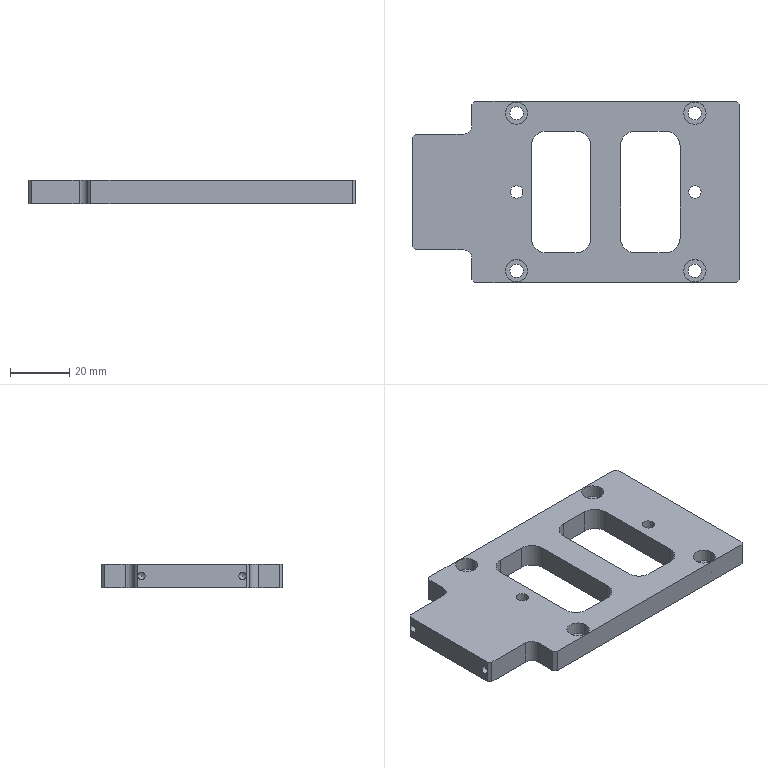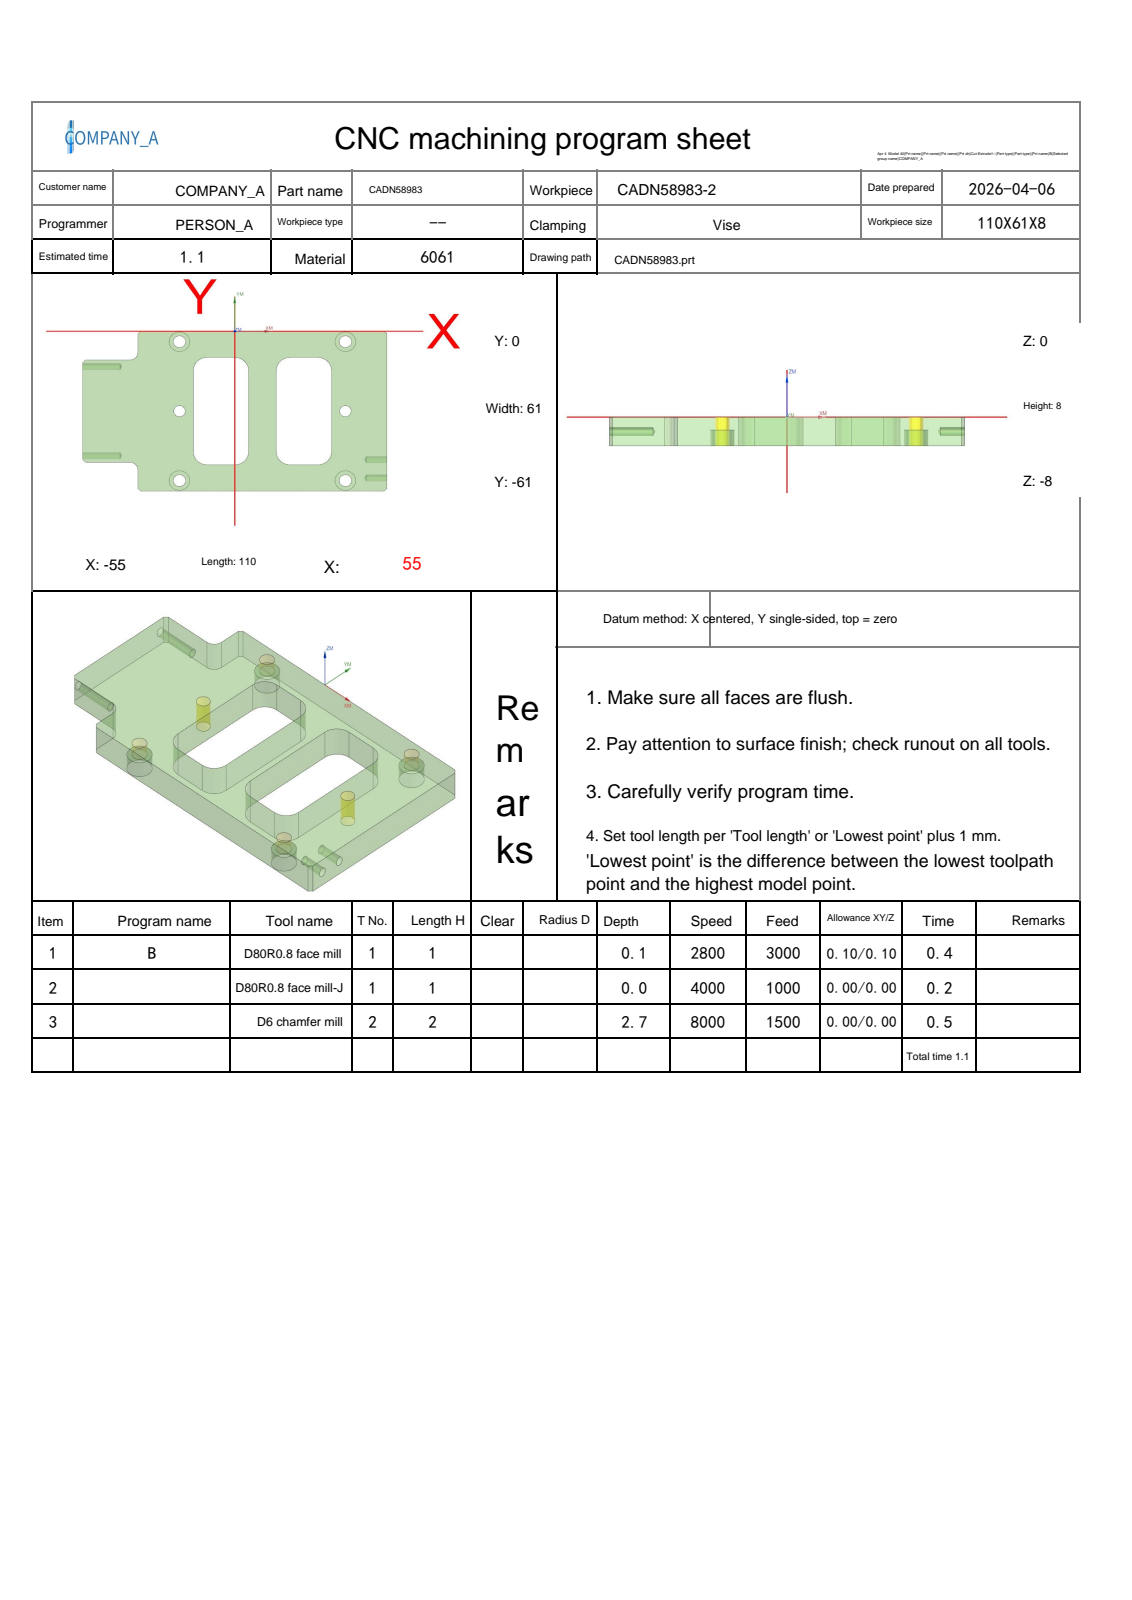NC program | NX | posted by the shop | part box 110 x 61 x 8 mm
Whole program:
%
O0001
(Machine time: 1.70 MIN)
(===Total Tool:2===)
(T1=D80R0.8 face mill D=80.  R=0.8  D-  H01 Z=0.    )
(T2=D6 chamfer mill   D=6.   R=0.   D-  H02 Z=-2.7  )
G80 G90 G17 G49 G40
G91 G28 Z0
M01
N1 T01 M06
(D80R0.8 face mill  D=80. R=0.8 H=01 ce=0.10 di=0.10)
G00 G90 G54 X107.097 Y-30.5 M03 S2800
G43 H01 Z20.
M08
Z3.525
G01 Z1.525 F3000.
X95.097
X-95.097
X-107.097
Z3.525
G00 X107.097
Z3.05
G01 Z1.05
X95.097
X-95.097
X-107.097
Z3.05
G00 X107.097
Z2.575
G01 Z.575
X95.097
X-95.097
X-107.097
Z2.575
G00 X107.097
Z2.1
G01 Z.1
X95.097
X-95.097
X-107.097
Z2.1
G00 Z20.
G91 G28 Z0.0
M05
M09
G91 G28 Z0.0
M01
N2 T01 M06
(D80R0.8 face mill-J  D=80. R=0.8 H=01 ce=0.00 di=0.00)
G00 G90 G54 X106.999 Y-30.5 M03 S4000
G43 H01 Z20.
M08
Z2.
G01 Z0.0 F1000.
X94.999
X-94.999
X-106.999
Z2.
G00 Z20.
G91 G28 Z0.0
M05
M09
G91 G28 Z0.0
M01
N3 T02 M06
(D6 chamfer mill  D=6. R=0. H=02 ce=0.00 di=0.00)
G00 G90 G54 X40. Y-30.5 M03 S8000
G43 H02 Z20.
M08
G98 G81 X40. Y-30.5 Z-2.7 R3. F1000.
X-20.
G80
G00 Z20.
G00 G90 X40. Y-57. M03 S8000
Z20.
G98 G81 X40. Y-57. Z-2.55 R3. F1000.
Y-4.
X-20.
Y-57.
G80
G00 Z20.
G00 G90 X10.386 Y-62.227 M03 S6500
Z20.
Z.172
G01 Z-1.2 F1500.
G03 X10.1 Y-62.027 I-1.286 J-1.532
G01 X10.054 Y-61.997
X10. Y-62.
X-34.
X-34.259 Y-61.966
X-34.5 Y-61.866
X-34.707 Y-61.707
X-35.707 Y-60.707
X-35.866 Y-60.5
X-35.966 Y-60.259
X-36. Y-60.
Y-53.
G03 X-38. Y-51. I-2. J0.0
G01 X-54.
X-54.259 Y-50.966
X-54.5 Y-50.866
X-54.707 Y-50.707
X-55.707 Y-49.707
X-55.866 Y-49.5
X-55.966 Y-49.259
X-56. Y-49.
Y-12.
X-55.966 Y-11.741
X-55.866 Y-11.5
X-55.707 Y-11.293
X-54.707 Y-10.293
X-54.5 Y-10.134
X-54.259 Y-10.034
X-54. Y-10.
X-38.
G03 X-36. Y-8. I0.0 J2.
G01 Y-1.
X-35.966 Y-.741
X-35.866 Y-.5
X-35.707 Y-.293
X-34.707 Y.707
X-34.5 Y.866
X-34.259 Y.966
X-34. Y1.
X54.
X54.259 Y.966
X54.5 Y.866
X54.707 Y.707
X55.707 Y-.293
X55.866 Y-.5
X55.966 Y-.741
X56. Y-1.
Y-60.
X55.966 Y-60.259
X55.866 Y-60.5
X55.707 Y-60.707
X54.707 Y-61.707
X54.5 Y-61.866
X54.259 Y-61.966
X54. Y-62.
X10.
X9.946 Y-61.997
X9.9 Y-62.027
G03 X9.614 Y-62.227 I1. J-1.732
G01 Z.172
G00 Z10.
X-21.065 Y-3.593
Z.294
G01 Z-1.2
G03 X-21.234 Y-3.898 I1.658 J-1.118
G01 X-21.259 Y-3.946
X-21.25 Y-4.
G03 X-20. Y-5.25 I1.25 J0.0
X-18.75 Y-4. I0.0 J1.25
X-20. Y-2.75 I-1.25 J0.0
X-21.223 Y-3.74 I0.0 J-1.25
G01 X-21.25 Y-4.
X-21.259 Y-4.054
X-21.234 Y-4.102
G03 X-21.065 Y-4.407 I1.827 J.813
G01 Z.294
G00 Z10.
X-19.074 Y-30.912
Z.32
G01 Z-1.2
G03 X-18.914 Y-30.603 I-1.687 J1.075
G01 X-18.89 Y-30.554
X-18.9 Y-30.5
G03 X-20. Y-29.4 I-1.1 J0.0
X-21.1 Y-30.5 I0.0 J-1.1
X-20. Y-31.6 I1.1 J0.0
X-18.9 Y-30.5 I0.0 J1.1
G01 X-18.89 Y-30.446
X-18.914 Y-30.397
G03 X-19.074 Y-30.088 I-1.848 J-.765
G01 Z.32
G00 Z10.
X-21.065 Y-56.593
Z.294
G01 Z-1.2
G03 X-21.234 Y-56.898 I1.658 J-1.118
G01 X-21.259 Y-56.946
X-21.25 Y-57.
G03 X-20. Y-58.25 I1.25 J0.0
X-18.75 Y-57. I0.0 J1.25
X-20. Y-55.75 I-1.25 J0.0
X-21.223 Y-56.74 I0.0 J-1.25
G01 X-21.25 Y-57.
X-21.259 Y-57.054
X-21.234 Y-57.102
G03 X-21.065 Y-57.407 I1.827 J.813
G01 Z.294
G00 Z10.
X3.773 Y-30.886
Z.172
G01 Z-1.2
G03 X3.973 Y-30.6 I-1.532 J1.286
G01 X4.003 Y-30.554
X4. Y-30.5
Y-15.
G03 X0.0 Y-11. I-4. J0.0
G01 X-10.
G03 X-14. Y-15. I0.0 J-4.
G01 Y-46.
G03 X-10. Y-50. I4. J0.0
G01 X0.0
G03 X4. Y-46. I0.0 J4.
G01 Y-30.5
X4.003 Y-30.446
X3.973 Y-30.4
G03 X3.773 Y-30.114 I-1.732 J-1.
G01 Z.172
G00 Z10.
X16.227
Z.172
G01 Z-1.2
G03 X16.027 Y-30.4 I1.532 J-1.286
G01 X15.997 Y-30.446
X16. Y-30.5
Y-46.
G03 X20. Y-50. I4. J0.0
G01 X30.
G03 X34. Y-46. I0.0 J4.
G01 Y-15.
G03 X30. Y-11. I-4. J0.0
G01 X20.
G03 X16. Y-15. I0.0 J-4.
G01 Y-30.5
X15.997 Y-30.554
X16.027 Y-30.6
G03 X16.227 Y-30.886 I1.732 J1.
G01 Z.172
G00 Z10.
X38.935 Y-56.593
Z.294
G01 Z-1.2
G03 X38.766 Y-56.898 I1.658 J-1.118
G01 X38.741 Y-56.946
X38.75 Y-57.
G03 X40. Y-58.25 I1.25 J0.0
X41.25 Y-57. I0.0 J1.25
X40. Y-55.75 I-1.25 J0.0
X38.777 Y-56.74 I0.0 J-1.25
G01 X38.75 Y-57.
X38.741 Y-57.054
X38.766 Y-57.102
G03 X38.935 Y-57.407 I1.827 J.813
G01 Z.294
G00 Z10.
X40.926 Y-30.912
Z.32
G01 Z-1.2
G03 X41.086 Y-30.603 I-1.687 J1.075
G01 X41.11 Y-30.554
X41.1 Y-30.5
G03 X40. Y-29.4 I-1.1 J0.0
X38.9 Y-30.5 I0.0 J-1.1
X40. Y-31.6 I1.1 J0.0
X41.1 Y-30.5 I0.0 J1.1
G01 X41.11 Y-30.446
X41.086 Y-30.397
G03 X40.926 Y-30.088 I-1.848 J-.765
G01 Z.32
G00 Z10.
X38.935 Y-3.593
Z.294
G01 Z-1.2
G03 X38.766 Y-3.898 I1.658 J-1.118
G01 X38.741 Y-3.946
X38.75 Y-4.
G03 X40. Y-5.25 I1.25 J0.0
X41.25 Y-4. I0.0 J1.25
X40. Y-2.75 I-1.25 J0.0
X38.777 Y-3.74 I0.0 J-1.25
G01 X38.75 Y-4.
X38.741 Y-4.054
X38.766 Y-4.102
G03 X38.935 Y-4.407 I1.827 J.813
G01 Z.294
G00 Z20.
M05
M09
G91 G28 Z0.0
G91 G28 Y0.0
M30
%